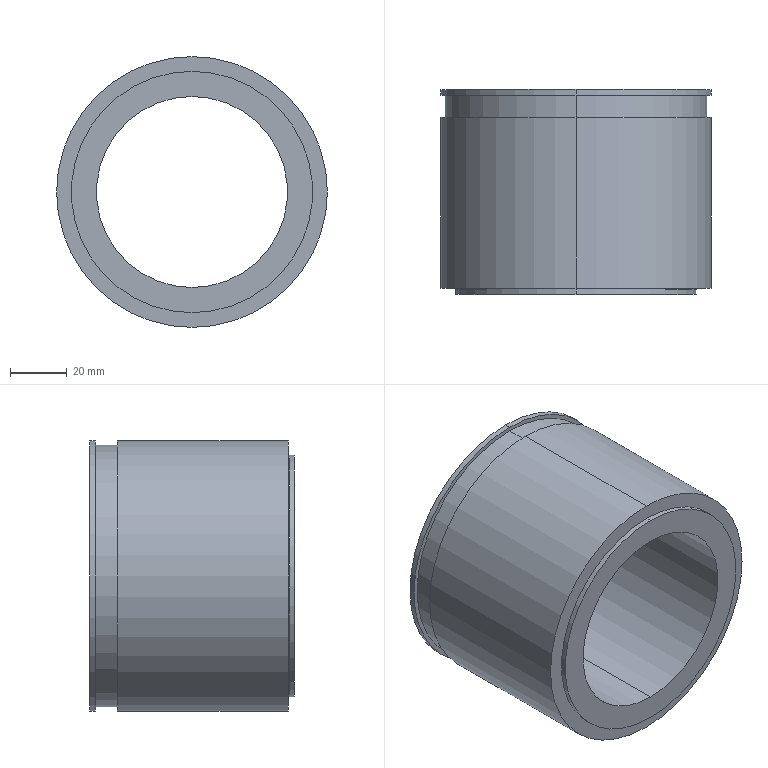Part | SolidWorks | features SavedExtBody 38 | 38 solids | 119 faces | box 95 x 71.846 x 95 mm | volume 199181 mm3 | sphere 72 | cylinder 26 | torus 12 | plane 9 | commonest cylinder face diameters 75.922 x6 79 x6 95 x4 67.029 x2 80 x2 83.136 x2